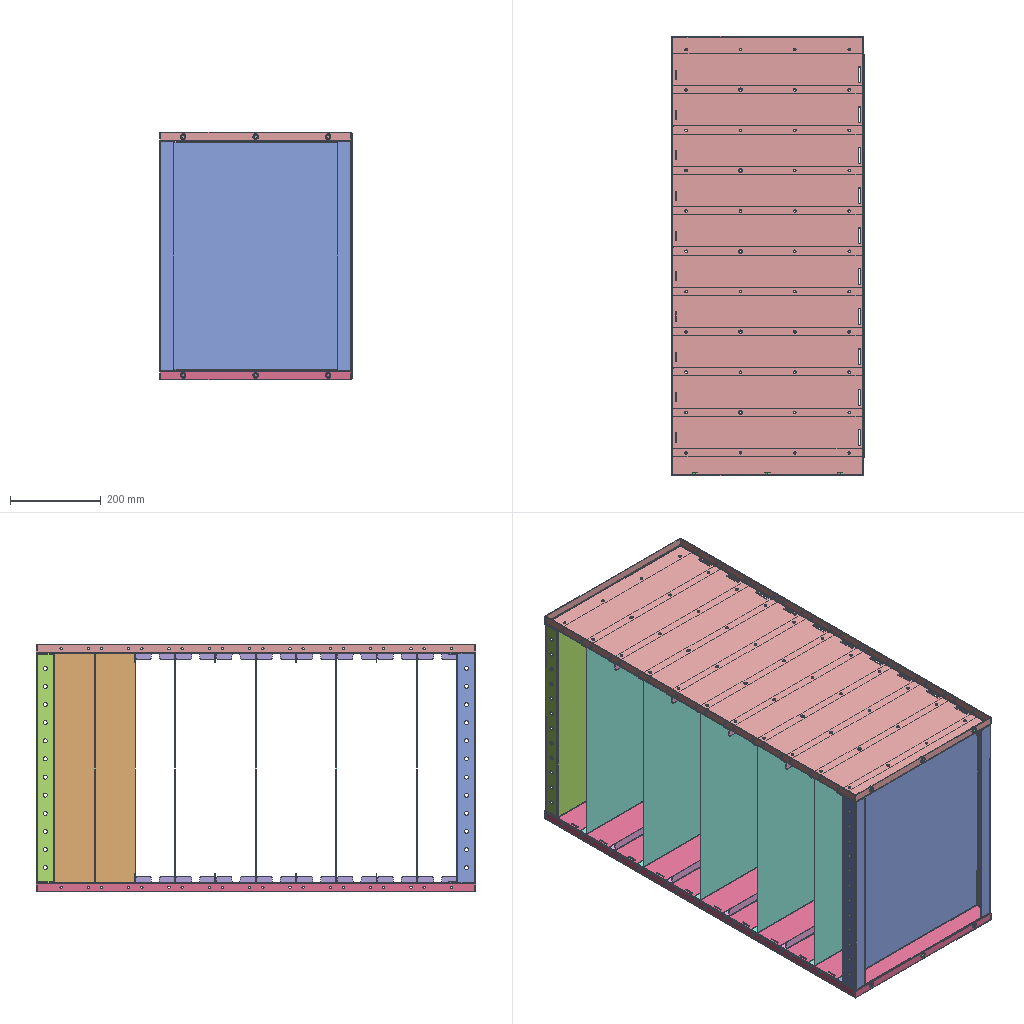Assembly | SolidWorks | 10 different items | 37 placed | box 425 x 970 x 547 mm
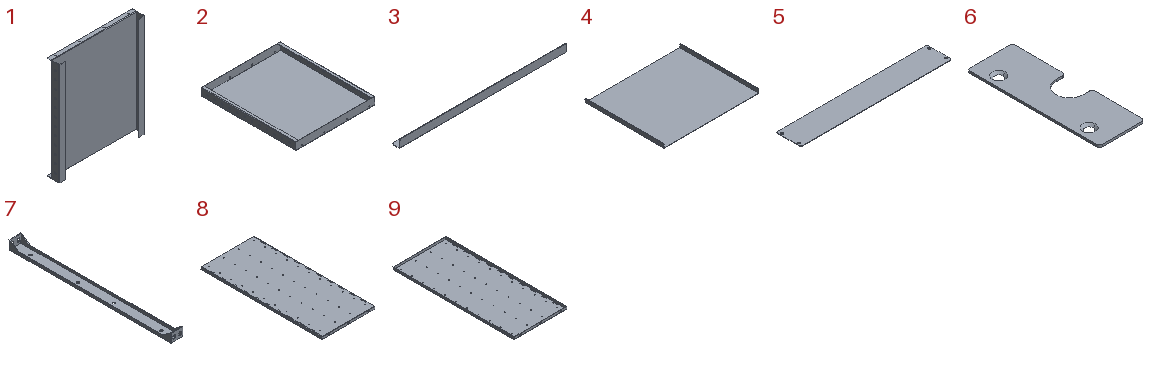Parts list (item | name | quantity | size | volume | features):
1 | - | x1 | 423 x 60 x 507 mm | 590095 mm3 | features BreakCorner 3, ICE 2, SMBaseFlange 2, Chamfer 1, EdgeFlange 1, FlatPattern 1, LPattern 1, MirrorPattern 1, SheetMetal 1
2 | - | x1 | 423 x 507 x 40 mm | 588577 mm3 | features ICE 3, EdgeFlange 2, Chamfer 1, CornerFeat 1, FlatPattern 1, LPattern 1, SMBaseFlange 1, SheetMetal 1
3 | - | x8 | 421 x 20 x 20 mm | 23768 mm3 | features Chamfer 1, EdgeFlange 1, Fillet 1, FlatPattern 1, ICE 1, LPattern 1, SMBaseFlange 1, SheetMetal 1
4 | - | x5 | 507 x 421 x 20 mm | 342480 mm3 | features Chamfer 1, EdgeFlange 1, Fillet 1, FlatPattern 1, ICE 1, SMBaseFlange 1, SheetMetal 1
5 | - | x2 | 541 x 88 x 1.5 mm | 71177 mm3 | features BreakCorner 1, Chamfer 1, FlatPattern 1, ICE 1, SMBaseFlange 1, SheetMetal 1
6 | - | x16 | 30 x 88 x 1.5 mm | 3479 mm3 | features Chamfer 1, Fillet 1, FlatPattern 1, ICE 1, SMBaseFlange 1, SheetMetal 1
7 | - | x1 | 40 x 545 x 30 mm | 65298 mm3 | features ICE 3, EdgeFlange 2, FlatPattern 1, SMBaseFlange 1, SheetMetal 1
8 | - | x1 | 423 x 970 x 20 mm | 908267 mm3 | features MirrorStock 1
9 | - | x1 | 423 x 970 x 20 mm | 908267 mm3 | features ICE 4, LPattern 4, CornerFeat 1, EdgeFlange 1, FlatPattern 1, SMBaseFlange 1, SheetMetal 1
10 | self-clinching nut_pmm | x1 | - | - | -
Mates (type | each side: item.copy, entity, surface, feature):
Coincident | 9.1 face plane Base-Flange1 | 1.1 face plane Edge-Flange1
Coincident | 9.1 face plane Edge-Flange1 | 1.1 face plane Base-Flange1
Coincident | 9.1 face plane Base-Flange1 | 2.1 face plane Edge-Flange1
Coincident | 9.1 face plane Edge-Flange1 | 2.1 face plane Edge-Flange1
Concentric | 9.1 face cylinder LPattern1 | 2.1 face cylinder Cut-Extrude1 | 2 times
Coincident | 9.1 face plane Base-Flange1 | 4.1 face plane Edge-Flange1
Coincident | 9.1 face plane Base-Flange1 | 3.1 face plane Base-Flange1
Concentric | 9.1 face cylinder LPattern1 | 4.1 edge
Concentric | 9.1 face cylinder LPattern1 | 4.1 face cone Chamfer1
Concentric | 9.1 face cylinder LPattern1 | 3.1 face cone Chamfer1 | 2 times
Concentric | 9.1 face cylinder LPattern4 | 5.1 face cone Chamfer1 | 2 times
Coincident | 9.1 face plane Edge-Flange1 | 6.1 face plane Base-Flange1
Concentric | 9.1 face cylinder Cut-Extrude4 | 6.1 face cone Chamfer1 | 2 times
Concentric | 6.2 face cone Chamfer1 | 8.1 face cylinder (H)PAXXX-LJ-08-20 Mirror | 2 times
Coincident | 6.1 face plane Base-Flange1 | 6.2 face plane Base-Flange1